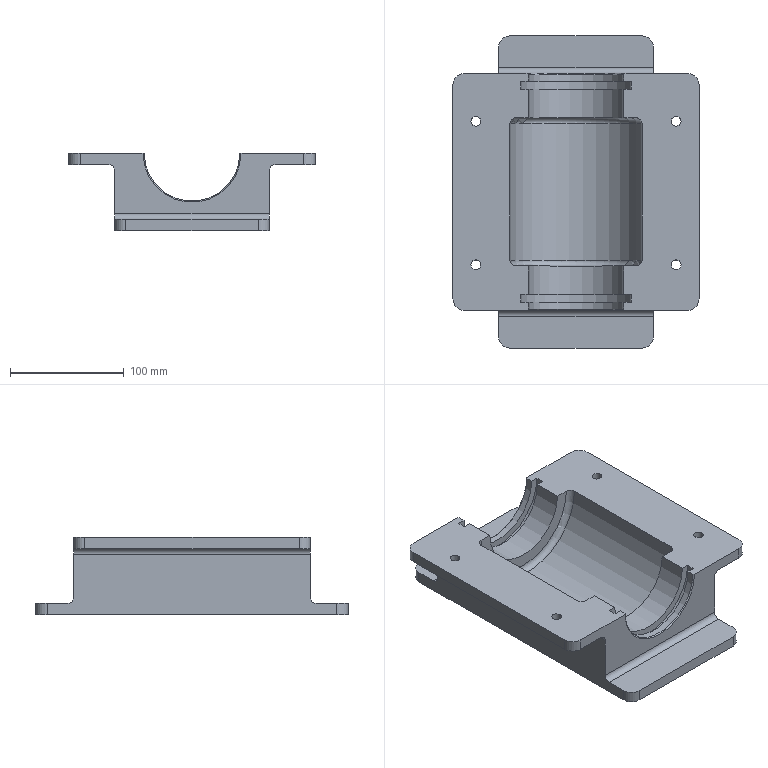Part | NX | features DATUM_CSYS 8, SKETCH 7, EXTRACT_FACE 4, HOLE PACKAGE 4, SIMPLE HOLE 4, SYMBOLIC_THREAD 4, Instance Feature 3, BLEND 2, EXTRUDE 2, CHAMFER 1, DATUM_PLANE 1, Pattern Feature 1, SWP104 1, UNITE 1 | 1 solid | 48 faces | box 216 x 274 x 68 mm | volume 1265227 mm3 | cylinder 23 | plane 21 | torus 2 | cone 2 | commonest cylinder face diameters 20 x8 8.5 x4 10 x4 84 x4 97 x2 116 x1
STEP:
#1=CARTESIAN_POINT('',(-24.25,199.,68.));
#2=VERTEX_POINT('',#1);
#3=CARTESIAN_POINT('',(-20.,199.,68.));
#4=DIRECTION('',(0.,0.,-1.));
#5=DIRECTION('',(-1.,0.,0.));
#6=AXIS2_PLACEMENT_3D('',#3,#4,#5);
#7=CIRCLE('',#6,4.25);
#8=EDGE_CURVE('',#2,#2,#7,.T.);
#9=ORIENTED_EDGE('',*,*,#8,.T.);
#10=EDGE_LOOP('',(#9));
#11=FACE_BOUND('',#10,.T.);
#12=CARTESIAN_POINT('',(-24.25,73.,68.));
#13=VERTEX_POINT('',#12);
#14=CARTESIAN_POINT('',(-20.,73.,68.));
#15=DIRECTION('',(0.,0.,-1.));
#16=DIRECTION('',(-1.,0.,0.));
#17=AXIS2_PLACEMENT_3D('',#14,#15,#16);
#18=CIRCLE('',#17,4.25);
#19=EDGE_CURVE('',#13,#13,#18,.T.);
#20=ORIENTED_EDGE('',*,*,#19,.T.);
#21=EDGE_LOOP('',(#20));
#22=FACE_BOUND('',#21,.T.);
#23=CARTESIAN_POINT('',(26.,240.,68.));
#24=VERTEX_POINT('',#23);
#25=CARTESIAN_POINT('',(26.,234.,68.));
#26=VERTEX_POINT('',#25);
#27=CARTESIAN_POINT('',(26.,33.,68.));
#28=DIRECTION('',(0.,-1.,0.));
#29=VECTOR('',#28,1000.);
#30=LINE('',#27,#29);
#31=EDGE_CURVE('',#24,#26,#30,.T.);
#32=ORIENTED_EDGE('',*,*,#31,.F.);
#33=CARTESIAN_POINT('',(25.,241.,68.));
#34=VERTEX_POINT('',#33);
#35=CARTESIAN_POINT('',(68.,198.,68.));
#36=DIRECTION('',(0.7071,-0.7071,0.));
#37=VECTOR('',#36,1000.);
#38=LINE('',#35,#37);
#39=EDGE_CURVE('',#24,#34,#38,.F.);
#40=ORIENTED_EDGE('',*,*,#39,.T.);
#41=CARTESIAN_POINT('',(-30.,241.,68.));
#42=VERTEX_POINT('',#41);
#43=CARTESIAN_POINT('',(176.,241.,68.));
#44=DIRECTION('',(-1.,0.,0.));
#45=VECTOR('',#44,1000.);
#46=LINE('',#43,#45);
#47=EDGE_CURVE('',#34,#42,#46,.T.);
#48=ORIENTED_EDGE('',*,*,#47,.T.);
#49=CARTESIAN_POINT('',(-40.,231.,68.));
#50=VERTEX_POINT('',#49);
#51=CARTESIAN_POINT('',(-30.,231.,68.));
#52=DIRECTION('',(0.,0.,1.));
#53=DIRECTION('',(1.,0.,0.));
#54=AXIS2_PLACEMENT_3D('',#51,#52,#53);
#55=CIRCLE('',#54,10.);
#56=EDGE_CURVE('',#42,#50,#55,.T.);
#57=ORIENTED_EDGE('',*,*,#56,.T.);
#58=CARTESIAN_POINT('',(-40.,43.,68.));
#59=VERTEX_POINT('',#58);
#60=CARTESIAN_POINT('',(-40.,241.,68.));
#61=DIRECTION('',(0.,-1.,0.));
#62=VECTOR('',#61,1000.);
#63=LINE('',#60,#62);
#64=EDGE_CURVE('',#50,#59,#63,.T.);
#65=ORIENTED_EDGE('',*,*,#64,.T.);
#66=CARTESIAN_POINT('',(-30.,33.,68.));
#67=VERTEX_POINT('',#66);
#68=CARTESIAN_POINT('',(-30.,43.,68.));
#69=DIRECTION('',(0.,0.,1.));
#70=DIRECTION('',(1.,0.,0.));
#71=AXIS2_PLACEMENT_3D('',#68,#69,#70);
#72=CIRCLE('',#71,10.);
#73=EDGE_CURVE('',#59,#67,#72,.T.);
#74=ORIENTED_EDGE('',*,*,#73,.T.);
#75=CARTESIAN_POINT('',(25.,33.,68.));
#76=VERTEX_POINT('',#75);
#77=CARTESIAN_POINT('',(176.,33.,68.));
#78=DIRECTION('',(-1.,0.,0.));
#79=VECTOR('',#78,1000.);
#80=LINE('',#77,#79);
#81=EDGE_CURVE('',#76,#67,#80,.T.);
#82=ORIENTED_EDGE('',*,*,#81,.F.);
#83=CARTESIAN_POINT('',(26.,34.,68.));
#84=VERTEX_POINT('',#83);
#85=CARTESIAN_POINT('',(68.,76.,68.));
#86=DIRECTION('',(-0.7071,-0.7071,0.));
#87=VECTOR('',#86,1000.);
#88=LINE('',#85,#87);
#89=EDGE_CURVE('',#76,#84,#88,.F.);
#90=ORIENTED_EDGE('',*,*,#89,.T.);
#91=CARTESIAN_POINT('',(26.,40.,68.));
#92=VERTEX_POINT('',#91);
#93=CARTESIAN_POINT('',(26.,33.,68.));
#94=DIRECTION('',(0.,-1.,0.));
#95=VECTOR('',#94,1000.);
#96=LINE('',#93,#95);
#97=EDGE_CURVE('',#92,#84,#96,.T.);
#98=ORIENTED_EDGE('',*,*,#97,.F.);
#99=CARTESIAN_POINT('',(19.5,40.,68.));
#100=VERTEX_POINT('',#99);
#101=CARTESIAN_POINT('',(176.,40.,68.));
#102=DIRECTION('',(1.,0.,0.));
#103=VECTOR('',#102,1000.);
#104=LINE('',#101,#103);
#105=EDGE_CURVE('',#100,#92,#104,.T.);
#106=ORIENTED_EDGE('',*,*,#105,.F.);
#107=CARTESIAN_POINT('',(19.5,47.,68.));
#108=VERTEX_POINT('',#107);
#109=CARTESIAN_POINT('',(19.5,33.,68.));
#110=DIRECTION('',(0.,-1.,0.));
#111=VECTOR('',#110,1000.);
#112=LINE('',#109,#111);
#113=EDGE_CURVE('',#108,#100,#112,.T.);
#114=ORIENTED_EDGE('',*,*,#113,.F.);
#115=CARTESIAN_POINT('',(26.,47.,68.));
#116=VERTEX_POINT('',#115);
#117=CARTESIAN_POINT('',(176.,47.,68.));
#118=DIRECTION('',(-1.,0.,0.));
#119=VECTOR('',#118,1000.);
#120=LINE('',#117,#119);
#121=EDGE_CURVE('',#116,#108,#120,.T.);
#122=ORIENTED_EDGE('',*,*,#121,.F.);
#123=CARTESIAN_POINT('',(26.,72.,68.));
#124=VERTEX_POINT('',#123);
#125=CARTESIAN_POINT('',(26.,33.,68.));
#126=DIRECTION('',(0.,-1.,0.));
#127=VECTOR('',#126,1000.);
#128=LINE('',#125,#127);
#129=EDGE_CURVE('',#124,#116,#128,.T.);
#130=ORIENTED_EDGE('',*,*,#129,.F.);
#131=CARTESIAN_POINT('',(15.,72.,68.));
#132=VERTEX_POINT('',#131);
#133=CARTESIAN_POINT('',(176.,72.,68.));
#134=DIRECTION('',(1.,0.,0.));
#135=VECTOR('',#134,1000.);
#136=LINE('',#133,#135);
#137=EDGE_CURVE('',#132,#124,#136,.T.);
#138=ORIENTED_EDGE('',*,*,#137,.F.);
#139=CARTESIAN_POINT('',(10.,77.,68.));
#140=VERTEX_POINT('',#139);
#141=CARTESIAN_POINT('',(15.,77.,68.));
#142=DIRECTION('',(0.,0.,1.));
#143=DIRECTION('',(1.,0.,0.));
#144=AXIS2_PLACEMENT_3D('',#141,#142,#143);
#145=CIRCLE('',#144,5.);
#146=EDGE_CURVE('',#132,#140,#145,.F.);
#147=ORIENTED_EDGE('',*,*,#146,.T.);
#148=CARTESIAN_POINT('',(10.,197.,68.));
#149=VERTEX_POINT('',#148);
#150=CARTESIAN_POINT('',(10.,33.,68.));
#151=DIRECTION('',(0.,-1.,0.));
#152=VECTOR('',#151,1000.);
#153=LINE('',#150,#152);
#154=EDGE_CURVE('',#149,#140,#153,.T.);
#155=ORIENTED_EDGE('',*,*,#154,.F.);
#156=CARTESIAN_POINT('',(15.,202.,68.));
#157=VERTEX_POINT('',#156);
#158=CARTESIAN_POINT('',(15.,197.,68.));
#159=DIRECTION('',(0.,0.,1.));
#160=DIRECTION('',(1.,0.,0.));
#161=AXIS2_PLACEMENT_3D('',#158,#159,#160);
#162=CIRCLE('',#161,5.);
#163=EDGE_CURVE('',#149,#157,#162,.F.);
#164=ORIENTED_EDGE('',*,*,#163,.T.);
#165=CARTESIAN_POINT('',(26.,202.,68.));
#166=VERTEX_POINT('',#165);
#167=CARTESIAN_POINT('',(176.,202.,68.));
#168=DIRECTION('',(-1.,0.,0.));
#169=VECTOR('',#168,1000.);
#170=LINE('',#167,#169);
#171=EDGE_CURVE('',#166,#157,#170,.T.);
#172=ORIENTED_EDGE('',*,*,#171,.F.);
#173=CARTESIAN_POINT('',(26.,227.,68.));
#174=VERTEX_POINT('',#173);
#175=CARTESIAN_POINT('',(26.,33.,68.));
#176=DIRECTION('',(0.,-1.,0.));
#177=VECTOR('',#176,1000.);
#178=LINE('',#175,#177);
#179=EDGE_CURVE('',#174,#166,#178,.T.);
#180=ORIENTED_EDGE('',*,*,#179,.F.);
#181=CARTESIAN_POINT('',(19.5,227.,68.));
#182=VERTEX_POINT('',#181);
#183=CARTESIAN_POINT('',(176.,227.,68.));
#184=DIRECTION('',(1.,0.,0.));
#185=VECTOR('',#184,1000.);
#186=LINE('',#183,#185);
#187=EDGE_CURVE('',#182,#174,#186,.T.);
#188=ORIENTED_EDGE('',*,*,#187,.F.);
#189=CARTESIAN_POINT('',(19.5,234.,68.));
#190=VERTEX_POINT('',#189);
#191=CARTESIAN_POINT('',(19.5,33.,68.));
#192=DIRECTION('',(0.,-1.,0.));
#193=VECTOR('',#192,1000.);
#194=LINE('',#191,#193);
#195=EDGE_CURVE('',#190,#182,#194,.T.);
#196=ORIENTED_EDGE('',*,*,#195,.F.);
#197=CARTESIAN_POINT('',(176.,234.,68.));
#198=DIRECTION('',(-1.,0.,0.));
#199=VECTOR('',#198,1000.);
#200=LINE('',#197,#199);
#201=EDGE_CURVE('',#26,#190,#200,.T.);
#202=ORIENTED_EDGE('',*,*,#201,.F.);
#203=EDGE_LOOP('',(#32,#40,#48,#57,#65,#74,#82,#90,#98,#106,#114,#122,#130,#138,#147,#155,#164,#172,#180,#188,#196,#202));
#204=FACE_BOUND('',#203,.T.);
#205=CARTESIAN_POINT('',(176.,241.,68.));
#206=DIRECTION('',(0.,0.,1.));
#207=DIRECTION('',(1.,0.,0.));
#208=AXIS2_PLACEMENT_3D('',#205,#206,#207);
#209=PLANE('',#208);
#210=ADVANCED_FACE('',(#11,#22,#204),#209,.T.);
#211=CARTESIAN_POINT('',(-40.,231.,58.));
#212=VERTEX_POINT('',#211);
#213=CARTESIAN_POINT('',(-40.,43.,58.));
#214=VERTEX_POINT('',#213);
#215=CARTESIAN_POINT('',(-40.,241.,58.));
#216=DIRECTION('',(0.,-1.,0.));
#217=VECTOR('',#216,1000.);
#218=LINE('',#215,#217);
#219=EDGE_CURVE('',#212,#214,#218,.T.);
#220=ORIENTED_EDGE('',*,*,#219,.T.);
#221=CARTESIAN_POINT('',(-40.,43.,68.));
#222=DIRECTION('',(0.,0.,-1.));
#223=VECTOR('',#222,1000.);
#224=LINE('',#221,#223);
#225=EDGE_CURVE('',#214,#59,#224,.F.);
#226=ORIENTED_EDGE('',*,*,#225,.T.);
#227=ORIENTED_EDGE('',*,*,#64,.F.);
#228=CARTESIAN_POINT('',(-40.,231.,58.));
#229=DIRECTION('',(0.,0.,-1.));
#230=VECTOR('',#229,1000.);
#231=LINE('',#228,#230);
#232=EDGE_CURVE('',#50,#212,#231,.T.);
#233=ORIENTED_EDGE('',*,*,#232,.T.);
#234=EDGE_LOOP('',(#220,#226,#227,#233));
#235=FACE_BOUND('',#234,.T.);
#236=CARTESIAN_POINT('',(-40.,241.,68.));
#237=DIRECTION('',(-1.,0.,0.));
#238=DIRECTION('',(0.,0.,1.));
#239=AXIS2_PLACEMENT_3D('',#236,#237,#238);
#240=PLANE('',#239);
#241=ADVANCED_FACE('',(#235),#240,.T.);
#242=CARTESIAN_POINT('',(-24.25,199.,58.));
#243=VERTEX_POINT('',#242);
#244=CARTESIAN_POINT('',(-20.,199.,58.));
#245=DIRECTION('',(0.,0.,-1.));
#246=DIRECTION('',(-1.,0.,0.));
#247=AXIS2_PLACEMENT_3D('',#244,#245,#246);
#248=CIRCLE('',#247,4.25);
#249=EDGE_CURVE('',#243,#243,#248,.T.);
#250=ORIENTED_EDGE('',*,*,#249,.F.);
#251=EDGE_LOOP('',(#250));
#252=FACE_BOUND('',#251,.T.);
#253=CARTESIAN_POINT('',(-24.25,73.,58.));
#254=VERTEX_POINT('',#253);
#255=CARTESIAN_POINT('',(-20.,73.,58.));
#256=DIRECTION('',(0.,0.,-1.));
#257=DIRECTION('',(-1.,0.,0.));
#258=AXIS2_PLACEMENT_3D('',#255,#256,#257);
#259=CIRCLE('',#258,4.25);
#260=EDGE_CURVE('',#254,#254,#259,.T.);
#261=ORIENTED_EDGE('',*,*,#260,.F.);
#262=EDGE_LOOP('',(#261));
#263=FACE_BOUND('',#262,.T.);
#264=CARTESIAN_POINT('',(-30.,241.,58.));
#265=VERTEX_POINT('',#264);
#266=CARTESIAN_POINT('',(-5.,241.,58.));
#267=VERTEX_POINT('',#266);
#268=CARTESIAN_POINT('',(-40.,241.,58.));
#269=DIRECTION('',(1.,0.,0.));
#270=VECTOR('',#269,1000.);
#271=LINE('',#268,#270);
#272=EDGE_CURVE('',#265,#267,#271,.T.);
#273=ORIENTED_EDGE('',*,*,#272,.T.);
#274=CARTESIAN_POINT('',(-5.,33.,58.));
#275=VERTEX_POINT('',#274);
#276=CARTESIAN_POINT('',(-5.,33.,58.));
#277=DIRECTION('',(0.,-1.,0.));
#278=VECTOR('',#277,1000.);
#279=LINE('',#276,#278);
#280=EDGE_CURVE('',#267,#275,#279,.T.);
#281=ORIENTED_EDGE('',*,*,#280,.T.);
#282=CARTESIAN_POINT('',(-30.,33.,58.));
#283=VERTEX_POINT('',#282);
#284=CARTESIAN_POINT('',(-40.,33.,58.));
#285=DIRECTION('',(1.,0.,0.));
#286=VECTOR('',#285,1000.);
#287=LINE('',#284,#286);
#288=EDGE_CURVE('',#283,#275,#287,.T.);
#289=ORIENTED_EDGE('',*,*,#288,.F.);
#290=CARTESIAN_POINT('',(-30.,43.,58.));
#291=DIRECTION('',(0.,0.,-1.));
#292=DIRECTION('',(-1.,0.,0.));
#293=AXIS2_PLACEMENT_3D('',#290,#291,#292);
#294=CIRCLE('',#293,10.);
#295=EDGE_CURVE('',#283,#214,#294,.T.);
#296=ORIENTED_EDGE('',*,*,#295,.T.);
#297=ORIENTED_EDGE('',*,*,#219,.F.);
#298=CARTESIAN_POINT('',(-30.,231.,58.));
#299=DIRECTION('',(0.,0.,-1.));
#300=DIRECTION('',(-1.,0.,0.));
#301=AXIS2_PLACEMENT_3D('',#298,#299,#300);
#302=CIRCLE('',#301,10.);
#303=EDGE_CURVE('',#212,#265,#302,.T.);
#304=ORIENTED_EDGE('',*,*,#303,.T.);
#305=EDGE_LOOP('',(#273,#281,#289,#296,#297,#304));
#306=FACE_BOUND('',#305,.T.);
#307=CARTESIAN_POINT('',(-40.,241.,58.));
#308=DIRECTION('',(0.,0.,-1.));
#309=DIRECTION('',(-1.,0.,0.));
#310=AXIS2_PLACEMENT_3D('',#307,#308,#309);
#311=PLANE('',#310);
#312=ADVANCED_FACE('',(#252,#263,#306),#311,.T.);
#313=CARTESIAN_POINT('',(0.,33.,53.));
#314=VERTEX_POINT('',#313);
#315=CARTESIAN_POINT('',(0.,33.,15.));
#316=VERTEX_POINT('',#315);
#317=CARTESIAN_POINT('',(0.,33.,58.));
#318=DIRECTION('',(0.,0.,-1.));
#319=VECTOR('',#318,1000.);
#320=LINE('',#317,#319);
#321=EDGE_CURVE('',#314,#316,#320,.T.);
#322=ORIENTED_EDGE('',*,*,#321,.F.);
#323=CARTESIAN_POINT('',(0.,241.,53.));
#324=VERTEX_POINT('',#323);
#325=CARTESIAN_POINT('',(0.,241.,53.));
#326=DIRECTION('',(0.,-1.,0.));
#327=VECTOR('',#326,1000.);
#328=LINE('',#325,#327);
#329=EDGE_CURVE('',#314,#324,#328,.F.);
#330=ORIENTED_EDGE('',*,*,#329,.T.);
#331=CARTESIAN_POINT('',(0.,241.,15.));
#332=VERTEX_POINT('',#331);
#333=CARTESIAN_POINT('',(0.,241.,58.));
#334=DIRECTION('',(0.,0.,-1.));
#335=VECTOR('',#334,1000.);
#336=LINE('',#333,#335);
#337=EDGE_CURVE('',#324,#332,#336,.T.);
#338=ORIENTED_EDGE('',*,*,#337,.T.);
#339=CARTESIAN_POINT('',(0.,246.,10.));
#340=VERTEX_POINT('',#339);
#341=CARTESIAN_POINT('',(0.,246.,15.));
#342=DIRECTION('',(-1.,0.,0.));
#343=DIRECTION('',(0.,0.,1.));
#344=AXIS2_PLACEMENT_3D('',#341,#342,#343);
#345=CIRCLE('',#344,5.);
#346=EDGE_CURVE('',#332,#340,#345,.F.);
#347=ORIENTED_EDGE('',*,*,#346,.T.);
#348=CARTESIAN_POINT('',(0.,264.,10.));
#349=VERTEX_POINT('',#348);
#350=CARTESIAN_POINT('',(0.,274.,10.));
#351=DIRECTION('',(0.,-1.,0.));
#352=VECTOR('',#351,1000.);
#353=LINE('',#350,#352);
#354=EDGE_CURVE('',#349,#340,#353,.T.);
#355=ORIENTED_EDGE('',*,*,#354,.F.);
#356=CARTESIAN_POINT('',(0.,264.,0.));
#357=VERTEX_POINT('',#356);
#358=CARTESIAN_POINT('',(0.,264.,0.));
#359=DIRECTION('',(0.,0.,-1.));
#360=VECTOR('',#359,1000.);
#361=LINE('',#358,#360);
#362=EDGE_CURVE('',#349,#357,#361,.T.);
#363=ORIENTED_EDGE('',*,*,#362,.T.);
#364=CARTESIAN_POINT('',(0.,10.,0.));
#365=VERTEX_POINT('',#364);
#366=CARTESIAN_POINT('',(0.,274.,0.));
#367=DIRECTION('',(0.,-1.,0.));
#368=VECTOR('',#367,1000.);
#369=LINE('',#366,#368);
#370=EDGE_CURVE('',#357,#365,#369,.T.);
#371=ORIENTED_EDGE('',*,*,#370,.T.);
#372=CARTESIAN_POINT('',(0.,10.,10.));
#373=VERTEX_POINT('',#372);
#374=CARTESIAN_POINT('',(0.,10.,10.));
#375=DIRECTION('',(0.,0.,-1.));
#376=VECTOR('',#375,1000.);
#377=LINE('',#374,#376);
#378=EDGE_CURVE('',#365,#373,#377,.F.);
#379=ORIENTED_EDGE('',*,*,#378,.T.);
#380=CARTESIAN_POINT('',(0.,28.,10.));
#381=VERTEX_POINT('',#380);
#382=CARTESIAN_POINT('',(0.,274.,10.));
#383=DIRECTION('',(0.,-1.,0.));
#384=VECTOR('',#383,1000.);
#385=LINE('',#382,#384);
#386=EDGE_CURVE('',#381,#373,#385,.T.);
#387=ORIENTED_EDGE('',*,*,#386,.F.);
#388=CARTESIAN_POINT('',(0.,28.,15.));
#389=DIRECTION('',(-1.,0.,0.));
#390=DIRECTION('',(0.,0.,1.));
#391=AXIS2_PLACEMENT_3D('',#388,#389,#390);
#392=CIRCLE('',#391,5.);
#393=EDGE_CURVE('',#381,#316,#392,.F.);
#394=ORIENTED_EDGE('',*,*,#393,.T.);
#395=EDGE_LOOP('',(#322,#330,#338,#347,#355,#363,#371,#379,#387,#394));
#396=FACE_BOUND('',#395,.T.);
#397=CARTESIAN_POINT('',(0.,241.,58.));
#398=DIRECTION('',(-1.,0.,0.));
#399=DIRECTION('',(0.,0.,1.));
#400=AXIS2_PLACEMENT_3D('',#397,#398,#399);
#401=PLANE('',#400);
#402=ADVANCED_FACE('',(#396),#401,.T.);
#403=CARTESIAN_POINT('',(136.,241.,15.));
#404=VERTEX_POINT('',#403);
#405=CARTESIAN_POINT('',(136.,241.,53.));
#406=VERTEX_POINT('',#405);
#407=CARTESIAN_POINT('',(136.,241.,10.));
#408=DIRECTION('',(0.,0.,1.));
#409=VECTOR('',#408,1000.);
#410=LINE('',#407,#409);
#411=EDGE_CURVE('',#404,#406,#410,.T.);
#412=ORIENTED_EDGE('',*,*,#411,.T.);
#413=CARTESIAN_POINT('',(136.,33.,53.));
#414=VERTEX_POINT('',#413);
#415=CARTESIAN_POINT('',(136.,33.,53.));
#416=DIRECTION('',(0.,-1.,0.));
#417=VECTOR('',#416,1000.);
#418=LINE('',#415,#417);
#419=EDGE_CURVE('',#406,#414,#418,.T.);
#420=ORIENTED_EDGE('',*,*,#419,.T.);
#421=CARTESIAN_POINT('',(136.,33.,15.));
#422=VERTEX_POINT('',#421);
#423=CARTESIAN_POINT('',(136.,33.,10.));
#424=DIRECTION('',(0.,0.,1.));
#425=VECTOR('',#424,1000.);
#426=LINE('',#423,#425);
#427=EDGE_CURVE('',#422,#414,#426,.T.);
#428=ORIENTED_EDGE('',*,*,#427,.F.);
#429=CARTESIAN_POINT('',(136.,28.,10.));
#430=VERTEX_POINT('',#429);
#431=CARTESIAN_POINT('',(136.,28.,15.));
#432=DIRECTION('',(1.,0.,0.));
#433=DIRECTION('',(0.,0.,-1.));
#434=AXIS2_PLACEMENT_3D('',#431,#432,#433);
#435=CIRCLE('',#434,5.);
#436=EDGE_CURVE('',#422,#430,#435,.F.);
#437=ORIENTED_EDGE('',*,*,#436,.T.);
#438=CARTESIAN_POINT('',(136.,10.,10.));
#439=VERTEX_POINT('',#438);
#440=CARTESIAN_POINT('',(136.,0.,10.));
#441=DIRECTION('',(0.,1.,0.));
#442=VECTOR('',#441,1000.);
#443=LINE('',#440,#442);
#444=EDGE_CURVE('',#439,#430,#443,.T.);
#445=ORIENTED_EDGE('',*,*,#444,.F.);
#446=CARTESIAN_POINT('',(136.,10.,0.));
#447=VERTEX_POINT('',#446);
#448=CARTESIAN_POINT('',(136.,10.,0.));
#449=DIRECTION('',(0.,0.,-1.));
#450=VECTOR('',#449,1000.);
#451=LINE('',#448,#450);
#452=EDGE_CURVE('',#439,#447,#451,.T.);
#453=ORIENTED_EDGE('',*,*,#452,.T.);
#454=CARTESIAN_POINT('',(136.,264.,0.));
#455=VERTEX_POINT('',#454);
#456=CARTESIAN_POINT('',(136.,0.,0.));
#457=DIRECTION('',(0.,1.,0.));
#458=VECTOR('',#457,1000.);
#459=LINE('',#456,#458);
#460=EDGE_CURVE('',#447,#455,#459,.T.);
#461=ORIENTED_EDGE('',*,*,#460,.T.);
#462=CARTESIAN_POINT('',(136.,264.,10.));
#463=VERTEX_POINT('',#462);
#464=CARTESIAN_POINT('',(136.,264.,10.));
#465=DIRECTION('',(0.,0.,-1.));
#466=VECTOR('',#465,1000.);
#467=LINE('',#464,#466);
#468=EDGE_CURVE('',#455,#463,#467,.F.);
#469=ORIENTED_EDGE('',*,*,#468,.T.);
#470=CARTESIAN_POINT('',(136.,246.,10.));
#471=VERTEX_POINT('',#470);
#472=CARTESIAN_POINT('',(136.,0.,10.));
#473=DIRECTION('',(0.,1.,0.));
#474=VECTOR('',#473,1000.);
#475=LINE('',#472,#474);
#476=EDGE_CURVE('',#471,#463,#475,.T.);
#477=ORIENTED_EDGE('',*,*,#476,.F.);
#478=CARTESIAN_POINT('',(136.,246.,15.));
#479=DIRECTION('',(1.,0.,0.));
#480=DIRECTION('',(0.,0.,-1.));
#481=AXIS2_PLACEMENT_3D('',#478,#479,#480);
#482=CIRCLE('',#481,5.);
#483=EDGE_CURVE('',#471,#404,#482,.F.);
#484=ORIENTED_EDGE('',*,*,#483,.T.);
#485=EDGE_LOOP('',(#412,#420,#428,#437,#445,#453,#461,#469,#477,#484));
#486=FACE_BOUND('',#485,.T.);
#487=CARTESIAN_POINT('',(136.,241.,10.));
#488=DIRECTION('',(1.,0.,0.));
#489=DIRECTION('',(0.,0.,-1.));
#490=AXIS2_PLACEMENT_3D('',#487,#488,#489);
#491=PLANE('',#490);
#492=ADVANCED_FACE('',(#486),#491,.T.);
#493=CARTESIAN_POINT('',(151.75,199.,58.));
#494=VERTEX_POINT('',#493);
#495=CARTESIAN_POINT('',(156.,199.,58.));
#496=DIRECTION('',(0.,0.,-1.));
#497=DIRECTION('',(-1.,0.,0.));
#498=AXIS2_PLACEMENT_3D('',#495,#496,#497);
#499=CIRCLE('',#498,4.25);
#500=EDGE_CURVE('',#494,#494,#499,.T.);
#501=ORIENTED_EDGE('',*,*,#500,.F.);
#502=EDGE_LOOP('',(#501));
#503=FACE_BOUND('',#502,.T.);
#504=CARTESIAN_POINT('',(151.75,73.,58.));
#505=VERTEX_POINT('',#504);
#506=CARTESIAN_POINT('',(156.,73.,58.));
#507=DIRECTION('',(0.,0.,-1.));
#508=DIRECTION('',(-1.,0.,0.));
#509=AXIS2_PLACEMENT_3D('',#506,#507,#508);
#510=CIRCLE('',#509,4.25);
#511=EDGE_CURVE('',#505,#505,#510,.T.);
#512=ORIENTED_EDGE('',*,*,#511,.F.);
#513=EDGE_LOOP('',(#512));
#514=FACE_BOUND('',#513,.T.);
#515=CARTESIAN_POINT('',(141.,33.,58.));
#516=VERTEX_POINT('',#515);
#517=CARTESIAN_POINT('',(166.,33.,58.));
#518=VERTEX_POINT('',#517);
#519=CARTESIAN_POINT('',(136.,33.,58.));
#520=DIRECTION('',(1.,0.,0.));
#521=VECTOR('',#520,1000.);
#522=LINE('',#519,#521);
#523=EDGE_CURVE('',#516,#518,#522,.T.);
#524=ORIENTED_EDGE('',*,*,#523,.F.);
#525=CARTESIAN_POINT('',(141.,241.,58.));
#526=VERTEX_POINT('',#525);
#527=CARTESIAN_POINT('',(141.,241.,58.));
#528=DIRECTION('',(0.,-1.,0.));
#529=VECTOR('',#528,1000.);
#530=LINE('',#527,#529);
#531=EDGE_CURVE('',#516,#526,#530,.F.);
#532=ORIENTED_EDGE('',*,*,#531,.T.);
#533=CARTESIAN_POINT('',(166.,241.,58.));
#534=VERTEX_POINT('',#533);
#535=CARTESIAN_POINT('',(136.,241.,58.));
#536=DIRECTION('',(1.,0.,0.));
#537=VECTOR('',#536,1000.);
#538=LINE('',#535,#537);
#539=EDGE_CURVE('',#526,#534,#538,.T.);
#540=ORIENTED_EDGE('',*,*,#539,.T.);
#541=CARTESIAN_POINT('',(176.,231.,58.));
#542=VERTEX_POINT('',#541);
#543=CARTESIAN_POINT('',(166.,231.,58.));
#544=DIRECTION('',(0.,0.,-1.));
#545=DIRECTION('',(-1.,0.,0.));
#546=AXIS2_PLACEMENT_3D('',#543,#544,#545);
#547=CIRCLE('',#546,10.);
#548=EDGE_CURVE('',#534,#542,#547,.T.);
#549=ORIENTED_EDGE('',*,*,#548,.T.);
#550=CARTESIAN_POINT('',(176.,43.,58.));
#551=VERTEX_POINT('',#550);
#552=CARTESIAN_POINT('',(176.,241.,58.));
#553=DIRECTION('',(0.,-1.,0.));
#554=VECTOR('',#553,1000.);
#555=LINE('',#552,#554);
#556=EDGE_CURVE('',#542,#551,#555,.T.);
#557=ORIENTED_EDGE('',*,*,#556,.T.);
#558=CARTESIAN_POINT('',(166.,43.,58.));
#559=DIRECTION('',(0.,0.,-1.));
#560=DIRECTION('',(-1.,0.,0.));
#561=AXIS2_PLACEMENT_3D('',#558,#559,#560);
#562=CIRCLE('',#561,10.);
#563=EDGE_CURVE('',#551,#518,#562,.T.);
#564=ORIENTED_EDGE('',*,*,#563,.T.);
#565=EDGE_LOOP('',(#524,#532,#540,#549,#557,#564));
#566=FACE_BOUND('',#565,.T.);
#567=CARTESIAN_POINT('',(136.,241.,58.));
#568=DIRECTION('',(0.,0.,-1.));
#569=DIRECTION('',(-1.,0.,0.));
#570=AXIS2_PLACEMENT_3D('',#567,#568,#569);
#571=PLANE('',#570);
#572=ADVANCED_FACE('',(#503,#514,#566),#571,.T.);
#573=CARTESIAN_POINT('',(176.,231.,68.));
#574=VERTEX_POINT('',#573);
#575=CARTESIAN_POINT('',(176.,43.,68.));
#576=VERTEX_POINT('',#575);
#577=CARTESIAN_POINT('',(176.,241.,68.));
#578=DIRECTION('',(0.,-1.,0.));
#579=VECTOR('',#578,1000.);
#580=LINE('',#577,#579);
#581=EDGE_CURVE('',#574,#576,#580,.T.);
#582=ORIENTED_EDGE('',*,*,#581,.T.);
#583=CARTESIAN_POINT('',(176.,43.,58.));
#584=DIRECTION('',(0.,0.,1.));
#585=VECTOR('',#584,1000.);
#586=LINE('',#583,#585);
#587=EDGE_CURVE('',#576,#551,#586,.F.);
#588=ORIENTED_EDGE('',*,*,#587,.T.);
#589=ORIENTED_EDGE('',*,*,#556,.F.);
#590=CARTESIAN_POINT('',(176.,231.,68.));
#591=DIRECTION('',(0.,0.,1.));
#592=VECTOR('',#591,1000.);
#593=LINE('',#590,#592);
#594=EDGE_CURVE('',#542,#574,#593,.T.);
#595=ORIENTED_EDGE('',*,*,#594,.T.);
#596=EDGE_LOOP('',(#582,#588,#589,#595));
#597=FACE_BOUND('',#596,.T.);
#598=CARTESIAN_POINT('',(176.,241.,58.));
#599=DIRECTION('',(1.,0.,0.));
#600=DIRECTION('',(0.,0.,-1.));
#601=AXIS2_PLACEMENT_3D('',#598,#599,#600);
#602=PLANE('',#601);
#603=ADVANCED_FACE('',(#597),#602,.T.);
#604=CARTESIAN_POINT('',(151.75,199.,68.));
#605=VERTEX_POINT('',#604);
#606=CARTESIAN_POINT('',(156.,199.,68.));
#607=DIRECTION('',(0.,0.,-1.));
#608=DIRECTION('',(-1.,0.,0.));
#609=AXIS2_PLACEMENT_3D('',#606,#607,#608);
#610=CIRCLE('',#609,4.25);
#611=EDGE_CURVE('',#605,#605,#610,.T.);
#612=ORIENTED_EDGE('',*,*,#611,.T.);
#613=EDGE_LOOP('',(#612));
#614=FACE_BOUND('',#613,.T.);
#615=CARTESIAN_POINT('',(151.75,73.,68.));
#616=VERTEX_POINT('',#615);
#617=CARTESIAN_POINT('',(156.,73.,68.));
#618=DIRECTION('',(0.,0.,-1.));
#619=DIRECTION('',(-1.,0.,0.));
#620=AXIS2_PLACEMENT_3D('',#617,#618,#619);
#621=CIRCLE('',#620,4.25);
#622=EDGE_CURVE('',#616,#616,#621,.T.);
#623=ORIENTED_EDGE('',*,*,#622,.T.);
#624=EDGE_LOOP('',(#623));
#625=FACE_BOUND('',#624,.T.);
#626=CARTESIAN_POINT('',(166.,241.,68.));
#627=VERTEX_POINT('',#626);
#628=CARTESIAN_POINT('',(111.,241.,68.));
#629=VERTEX_POINT('',#628);
#630=CARTESIAN_POINT('',(176.,241.,68.));
#631=DIRECTION('',(-1.,0.,0.));
#632=VECTOR('',#631,1000.);
#633=LINE('',#630,#632);
#634=EDGE_CURVE('',#627,#629,#633,.T.);
#635=ORIENTED_EDGE('',*,*,#634,.T.);
#636=CARTESIAN_POINT('',(110.,240.,68.));
#637=VERTEX_POINT('',#636);
#638=CARTESIAN_POINT('',(68.,198.,68.));
#639=DIRECTION('',(0.7071,0.7071,0.));
#640=VECTOR('',#639,1000.);
#641=LINE('',#638,#640);
#642=EDGE_CURVE('',#629,#637,#641,.F.);
#643=ORIENTED_EDGE('',*,*,#642,.T.);
#644=CARTESIAN_POINT('',(110.,234.,68.));
#645=VERTEX_POINT('',#644);
#646=CARTESIAN_POINT('',(110.,33.,68.));
#647=DIRECTION('',(0.,-1.,0.));
#648=VECTOR('',#647,1000.);
#649=LINE('',#646,#648);
#650=EDGE_CURVE('',#645,#637,#649,.F.);
#651=ORIENTED_EDGE('',*,*,#650,.F.);
#652=CARTESIAN_POINT('',(116.5,234.,68.));
#653=VERTEX_POINT('',#652);
#654=CARTESIAN_POINT('',(176.,234.,68.));
#655=DIRECTION('',(-1.,0.,0.));
#656=VECTOR('',#655,1000.);
#657=LINE('',#654,#656);
#658=EDGE_CURVE('',#653,#645,#657,.T.);
#659=ORIENTED_EDGE('',*,*,#658,.F.);
#660=CARTESIAN_POINT('',(116.5,227.,68.));
#661=VERTEX_POINT('',#660);
#662=CARTESIAN_POINT('',(116.5,33.,68.));
#663=DIRECTION('',(0.,-1.,0.));
#664=VECTOR('',#663,1000.);
#665=LINE('',#662,#664);
#666=EDGE_CURVE('',#661,#653,#665,.F.);
#667=ORIENTED_EDGE('',*,*,#666,.F.);
#668=CARTESIAN_POINT('',(110.,227.,68.));
#669=VERTEX_POINT('',#668);
#670=CARTESIAN_POINT('',(176.,227.,68.));
#671=DIRECTION('',(1.,0.,0.));
#672=VECTOR('',#671,1000.);
#673=LINE('',#670,#672);
#674=EDGE_CURVE('',#669,#661,#673,.T.);
#675=ORIENTED_EDGE('',*,*,#674,.F.);
#676=CARTESIAN_POINT('',(110.,202.,68.));
#677=VERTEX_POINT('',#676);
#678=CARTESIAN_POINT('',(110.,33.,68.));
#679=DIRECTION('',(0.,-1.,0.));
#680=VECTOR('',#679,1000.);
#681=LINE('',#678,#680);
#682=EDGE_CURVE('',#677,#669,#681,.F.);
#683=ORIENTED_EDGE('',*,*,#682,.F.);
#684=CARTESIAN_POINT('',(121.,202.,68.));
#685=VERTEX_POINT('',#684);
#686=CARTESIAN_POINT('',(176.,202.,68.));
#687=DIRECTION('',(-1.,0.,0.));
#688=VECTOR('',#687,1000.);
#689=LINE('',#686,#688);
#690=EDGE_CURVE('',#685,#677,#689,.T.);
#691=ORIENTED_EDGE('',*,*,#690,.F.);
#692=CARTESIAN_POINT('',(126.,197.,68.));
#693=VERTEX_POINT('',#692);
#694=CARTESIAN_POINT('',(121.,197.,68.));
#695=DIRECTION('',(0.,0.,1.));
#696=DIRECTION('',(1.,0.,0.));
#697=AXIS2_PLACEMENT_3D('',#694,#695,#696);
#698=CIRCLE('',#697,5.);
#699=EDGE_CURVE('',#685,#693,#698,.F.);
#700=ORIENTED_EDGE('',*,*,#699,.T.);
#701=CARTESIAN_POINT('',(126.,77.,68.));
#702=VERTEX_POINT('',#701);
#703=CARTESIAN_POINT('',(126.,33.,68.));
#704=DIRECTION('',(0.,-1.,0.));
#705=VECTOR('',#704,1000.);
#706=LINE('',#703,#705);
#707=EDGE_CURVE('',#702,#693,#706,.F.);
#708=ORIENTED_EDGE('',*,*,#707,.F.);
#709=CARTESIAN_POINT('',(121.,72.,68.));
#710=VERTEX_POINT('',#709);
#711=CARTESIAN_POINT('',(121.,77.,68.));
#712=DIRECTION('',(0.,0.,1.));
#713=DIRECTION('',(1.,0.,0.));
#714=AXIS2_PLACEMENT_3D('',#711,#712,#713);
#715=CIRCLE('',#714,5.);
#716=EDGE_CURVE('',#702,#710,#715,.F.);
#717=ORIENTED_EDGE('',*,*,#716,.T.);
#718=CARTESIAN_POINT('',(110.,72.,68.));
#719=VERTEX_POINT('',#718);
#720=CARTESIAN_POINT('',(176.,72.,68.));
#721=DIRECTION('',(1.,0.,0.));
#722=VECTOR('',#721,1000.);
#723=LINE('',#720,#722);
#724=EDGE_CURVE('',#719,#710,#723,.T.);
#725=ORIENTED_EDGE('',*,*,#724,.F.);
#726=CARTESIAN_POINT('',(110.,47.,68.));
#727=VERTEX_POINT('',#726);
#728=CARTESIAN_POINT('',(110.,33.,68.));
#729=DIRECTION('',(0.,-1.,0.));
#730=VECTOR('',#729,1000.);
#731=LINE('',#728,#730);
#732=EDGE_CURVE('',#727,#719,#731,.F.);
#733=ORIENTED_EDGE('',*,*,#732,.F.);
#734=CARTESIAN_POINT('',(116.5,47.,68.));
#735=VERTEX_POINT('',#734);
#736=CARTESIAN_POINT('',(176.,47.,68.));
#737=DIRECTION('',(-1.,0.,0.));
#738=VECTOR('',#737,1000.);
#739=LINE('',#736,#738);
#740=EDGE_CURVE('',#735,#727,#739,.T.);
#741=ORIENTED_EDGE('',*,*,#740,.F.);
#742=CARTESIAN_POINT('',(116.5,40.,68.));
#743=VERTEX_POINT('',#742);
#744=CARTESIAN_POINT('',(116.5,33.,68.));
#745=DIRECTION('',(0.,-1.,0.));
#746=VECTOR('',#745,1000.);
#747=LINE('',#744,#746);
#748=EDGE_CURVE('',#743,#735,#747,.F.);
#749=ORIENTED_EDGE('',*,*,#748,.F.);
#750=CARTESIAN_POINT('',(110.,40.,68.));
#751=VERTEX_POINT('',#750);
#752=CARTESIAN_POINT('',(176.,40.,68.));
#753=DIRECTION('',(1.,0.,0.));
#754=VECTOR('',#753,1000.);
#755=LINE('',#752,#754);
#756=EDGE_CURVE('',#751,#743,#755,.T.);
#757=ORIENTED_EDGE('',*,*,#756,.F.);
#758=CARTESIAN_POINT('',(110.,34.,68.));
#759=VERTEX_POINT('',#758);
#760=CARTESIAN_POINT('',(110.,33.,68.));
#761=DIRECTION('',(0.,-1.,0.));
#762=VECTOR('',#761,1000.);
#763=LINE('',#760,#762);
#764=EDGE_CURVE('',#759,#751,#763,.F.);
#765=ORIENTED_EDGE('',*,*,#764,.F.);
#766=CARTESIAN_POINT('',(111.,33.,68.));
#767=VERTEX_POINT('',#766);
#768=CARTESIAN_POINT('',(68.,76.,68.));
#769=DIRECTION('',(-0.7071,0.7071,0.));
#770=VECTOR('',#769,1000.);
#771=LINE('',#768,#770);
#772=EDGE_CURVE('',#759,#767,#771,.F.);
#773=ORIENTED_EDGE('',*,*,#772,.T.);
#774=CARTESIAN_POINT('',(166.,33.,68.));
#775=VERTEX_POINT('',#774);
#776=CARTESIAN_POINT('',(176.,33.,68.));
#777=DIRECTION('',(-1.,0.,0.));
#778=VECTOR('',#777,1000.);
#779=LINE('',#776,#778);
#780=EDGE_CURVE('',#775,#767,#779,.T.);
#781=ORIENTED_EDGE('',*,*,#780,.F.);
#782=CARTESIAN_POINT('',(166.,43.,68.));
#783=DIRECTION('',(0.,0.,1.));
#784=DIRECTION('',(1.,0.,0.));
#785=AXIS2_PLACEMENT_3D('',#782,#783,#784);
#786=CIRCLE('',#785,10.);
#787=EDGE_CURVE('',#775,#576,#786,.T.);
#788=ORIENTED_EDGE('',*,*,#787,.T.);
#789=ORIENTED_EDGE('',*,*,#581,.F.);
#790=CARTESIAN_POINT('',(166.,231.,68.));
#791=DIRECTION('',(0.,0.,1.));
#792=DIRECTION('',(1.,0.,0.));
#793=AXIS2_PLACEMENT_3D('',#790,#791,#792);
#794=CIRCLE('',#793,10.);
#795=EDGE_CURVE('',#574,#627,#794,.T.);
#796=ORIENTED_EDGE('',*,*,#795,.T.);
#797=EDGE_LOOP('',(#635,#643,#651,#659,#667,#675,#683,#691,#700,#708,#717,#725,#733,#741,#749,#757,#765,#773,#781,#788,#789,#796));
#798=FACE_BOUND('',#797,.T.);
#799=CARTESIAN_POINT('',(176.,241.,68.));
#800=DIRECTION('',(0.,0.,1.));
#801=DIRECTION('',(1.,0.,0.));
#802=AXIS2_PLACEMENT_3D('',#799,#800,#801);
#803=PLANE('',#802);
#804=ADVANCED_FACE('',(#614,#625,#798),#803,.T.);
#805=ORIENTED_EDGE('',*,*,#47,.F.);
#806=CARTESIAN_POINT('',(68.,241.,68.));
#807=DIRECTION('',(0.,-1.,0.));
#808=DIRECTION('',(0.,0.,-1.));
#809=AXIS2_PLACEMENT_3D('',#806,#807,#808);
#810=CIRCLE('',#809,43.);
#811=EDGE_CURVE('',#34,#629,#810,.T.);
#812=ORIENTED_EDGE('',*,*,#811,.T.);
#813=ORIENTED_EDGE('',*,*,#634,.F.);
#814=CARTESIAN_POINT('',(166.,241.,58.));
#815=DIRECTION('',(0.,0.,1.));
#816=VECTOR('',#815,1000.);
#817=LINE('',#814,#816);
#818=EDGE_CURVE('',#627,#534,#817,.F.);
#819=ORIENTED_EDGE('',*,*,#818,.T.);
#820=ORIENTED_EDGE('',*,*,#539,.F.);
#821=CARTESIAN_POINT('',(141.,241.,53.));
#822=DIRECTION('',(0.,-1.,0.));
#823=DIRECTION('',(0.,0.,-1.));
#824=AXIS2_PLACEMENT_3D('',#821,#822,#823);
#825=CIRCLE('',#824,5.);
#826=EDGE_CURVE('',#526,#406,#825,.T.);
#827=ORIENTED_EDGE('',*,*,#826,.T.);
#828=ORIENTED_EDGE('',*,*,#411,.F.);
#829=CARTESIAN_POINT('',(0.,241.,15.));
#830=DIRECTION('',(1.,0.,0.));
#831=VECTOR('',#830,1000.);
#832=LINE('',#829,#831);
#833=EDGE_CURVE('',#404,#332,#832,.F.);
#834=ORIENTED_EDGE('',*,*,#833,.T.);
#835=ORIENTED_EDGE('',*,*,#337,.F.);
#836=CARTESIAN_POINT('',(-5.,241.,53.));
#837=DIRECTION('',(0.,-1.,0.));
#838=DIRECTION('',(0.,0.,-1.));
#839=AXIS2_PLACEMENT_3D('',#836,#837,#838);
#840=CIRCLE('',#839,5.);
#841=EDGE_CURVE('',#324,#267,#840,.T.);
#842=ORIENTED_EDGE('',*,*,#841,.T.);
#843=ORIENTED_EDGE('',*,*,#272,.F.);
#844=CARTESIAN_POINT('',(-30.,241.,68.));
#845=DIRECTION('',(0.,0.,-1.));
#846=VECTOR('',#845,1000.);
#847=LINE('',#844,#846);
#848=EDGE_CURVE('',#265,#42,#847,.F.);
#849=ORIENTED_EDGE('',*,*,#848,.T.);
#850=EDGE_LOOP('',(#805,#812,#813,#819,#820,#827,#828,#834,#835,#842,#843,#849));
#851=FACE_BOUND('',#850,.T.);
#852=CARTESIAN_POINT('',(0.,241.,0.));
#853=DIRECTION('',(0.,-1.,0.));
#854=DIRECTION('',(0.,0.,-1.));
#855=AXIS2_PLACEMENT_3D('',#852,#853,#854);
#856=PLANE('',#855);
#857=ADVANCED_FACE('',(#851),#856,.F.);
#858=ORIENTED_EDGE('',*,*,#780,.T.);
#859=CARTESIAN_POINT('',(68.,33.,68.));
#860=DIRECTION('',(0.,-1.,0.));
#861=DIRECTION('',(0.,0.,-1.));
#862=AXIS2_PLACEMENT_3D('',#859,#860,#861);
#863=CIRCLE('',#862,43.);
#864=EDGE_CURVE('',#767,#76,#863,.F.);
#865=ORIENTED_EDGE('',*,*,#864,.T.);
#866=ORIENTED_EDGE('',*,*,#81,.T.);
#867=CARTESIAN_POINT('',(-30.,33.,0.));
#868=DIRECTION('',(0.,0.,-1.));
#869=VECTOR('',#868,1000.);
#870=LINE('',#867,#869);
#871=EDGE_CURVE('',#67,#283,#870,.T.);
#872=ORIENTED_EDGE('',*,*,#871,.T.);
#873=ORIENTED_EDGE('',*,*,#288,.T.);
#874=CARTESIAN_POINT('',(-5.,33.,53.));
#875=DIRECTION('',(0.,-1.,0.));
#876=DIRECTION('',(0.,0.,-1.));
#877=AXIS2_PLACEMENT_3D('',#874,#875,#876);
#878=CIRCLE('',#877,5.);
#879=EDGE_CURVE('',#275,#314,#878,.F.);
#880=ORIENTED_EDGE('',*,*,#879,.T.);
#881=ORIENTED_EDGE('',*,*,#321,.T.);
#882=CARTESIAN_POINT('',(136.,33.,15.));
#883=DIRECTION('',(1.,0.,0.));
#884=VECTOR('',#883,1000.);
#885=LINE('',#882,#884);
#886=EDGE_CURVE('',#316,#422,#885,.T.);
#887=ORIENTED_EDGE('',*,*,#886,.T.);
#888=ORIENTED_EDGE('',*,*,#427,.T.);
#889=CARTESIAN_POINT('',(141.,33.,53.));
#890=DIRECTION('',(0.,-1.,0.));
#891=DIRECTION('',(0.,0.,-1.));
#892=AXIS2_PLACEMENT_3D('',#889,#890,#891);
#893=CIRCLE('',#892,5.);
#894=EDGE_CURVE('',#414,#516,#893,.F.);
#895=ORIENTED_EDGE('',*,*,#894,.T.);
#896=ORIENTED_EDGE('',*,*,#523,.T.);
#897=CARTESIAN_POINT('',(166.,33.,0.));
#898=DIRECTION('',(0.,0.,1.));
#899=VECTOR('',#898,1000.);
#900=LINE('',#897,#899);
#901=EDGE_CURVE('',#518,#775,#900,.T.);
#902=ORIENTED_EDGE('',*,*,#901,.T.);
#903=EDGE_LOOP('',(#858,#865,#866,#872,#873,#880,#881,#887,#888,#895,#896,#902));
#904=FACE_BOUND('',#903,.T.);
#905=CARTESIAN_POINT('',(0.,33.,0.));
#906=DIRECTION('',(0.,-1.,0.));
#907=DIRECTION('',(0.,0.,-1.));
#908=AXIS2_PLACEMENT_3D('',#905,#906,#907);
#909=PLANE('',#908);
#910=ADVANCED_FACE('',(#904),#909,.T.);
#911=ORIENTED_EDGE('',*,*,#444,.T.);
#912=CARTESIAN_POINT('',(0.,28.,10.));
#913=DIRECTION('',(1.,0.,0.));
#914=VECTOR('',#913,1000.);
#915=LINE('',#912,#914);
#916=EDGE_CURVE('',#430,#381,#915,.F.);
#917=ORIENTED_EDGE('',*,*,#916,.T.);
#918=ORIENTED_EDGE('',*,*,#386,.T.);
#919=CARTESIAN_POINT('',(10.,0.,10.));
#920=VERTEX_POINT('',#919);
#921=CARTESIAN_POINT('',(10.,10.,10.));
#922=DIRECTION('',(0.,0.,1.));
#923=DIRECTION('',(1.,0.,0.));
#924=AXIS2_PLACEMENT_3D('',#921,#922,#923);
#925=CIRCLE('',#924,10.);
#926=EDGE_CURVE('',#373,#920,#925,.T.);
#927=ORIENTED_EDGE('',*,*,#926,.T.);
#928=CARTESIAN_POINT('',(126.,0.,10.));
#929=VERTEX_POINT('',#928);
#930=CARTESIAN_POINT('',(0.,0.,10.));
#931=DIRECTION('',(1.,0.,0.));
#932=VECTOR('',#931,1000.);
#933=LINE('',#930,#932);
#934=EDGE_CURVE('',#920,#929,#933,.T.);
#935=ORIENTED_EDGE('',*,*,#934,.T.);
#936=CARTESIAN_POINT('',(126.,10.,10.));
#937=DIRECTION('',(0.,0.,1.));
#938=DIRECTION('',(1.,0.,0.));
#939=AXIS2_PLACEMENT_3D('',#936,#937,#938);
#940=CIRCLE('',#939,10.);
#941=EDGE_CURVE('',#929,#439,#940,.T.);
#942=ORIENTED_EDGE('',*,*,#941,.T.);
#943=EDGE_LOOP('',(#911,#917,#918,#927,#935,#942));
#944=FACE_BOUND('',#943,.T.);
#945=CARTESIAN_POINT('',(0.,0.,10.));
#946=DIRECTION('',(0.,0.,1.));
#947=DIRECTION('',(1.,0.,0.));
#948=AXIS2_PLACEMENT_3D('',#945,#946,#947);
#949=PLANE('',#948);
#950=ADVANCED_FACE('',(#944),#949,.T.);
#951=CARTESIAN_POINT('',(10.,0.,0.));
#952=VERTEX_POINT('',#951);
#953=CARTESIAN_POINT('',(126.,0.,0.));
#954=VERTEX_POINT('',#953);
#955=CARTESIAN_POINT('',(0.,0.,0.));
#956=DIRECTION('',(1.,0.,0.));
#957=VECTOR('',#956,1000.);
#958=LINE('',#955,#957);
#959=EDGE_CURVE('',#952,#954,#958,.T.);
#960=ORIENTED_EDGE('',*,*,#959,.T.);
#961=CARTESIAN_POINT('',(126.,0.,10.));
#962=DIRECTION('',(0.,0.,-1.));
#963=VECTOR('',#962,1000.);
#964=LINE('',#961,#963);
#965=EDGE_CURVE('',#954,#929,#964,.F.);
#966=ORIENTED_EDGE('',*,*,#965,.T.);
#967=ORIENTED_EDGE('',*,*,#934,.F.);
#968=CARTESIAN_POINT('',(10.,0.,0.));
#969=DIRECTION('',(0.,0.,-1.));
#970=VECTOR('',#969,1000.);
#971=LINE('',#968,#970);
#972=EDGE_CURVE('',#920,#952,#971,.T.);
#973=ORIENTED_EDGE('',*,*,#972,.T.);
#974=EDGE_LOOP('',(#960,#966,#967,#973));
#975=FACE_BOUND('',#974,.T.);
#976=CARTESIAN_POINT('',(0.,0.,10.));
#977=DIRECTION('',(0.,1.,0.));
#978=DIRECTION('',(-1.,0.,0.));
#979=AXIS2_PLACEMENT_3D('',#976,#977,#978);
#980=PLANE('',#979);
#981=ADVANCED_FACE('',(#975),#980,.F.);
#982=CARTESIAN_POINT('',(126.,274.,0.));
#983=VERTEX_POINT('',#982);
#984=CARTESIAN_POINT('',(10.,274.,0.));
#985=VERTEX_POINT('',#984);
#986=CARTESIAN_POINT('',(136.,274.,0.));
#987=DIRECTION('',(-1.,0.,0.));
#988=VECTOR('',#987,1000.);
#989=LINE('',#986,#988);
#990=EDGE_CURVE('',#983,#985,#989,.T.);
#991=ORIENTED_EDGE('',*,*,#990,.T.);
#992=CARTESIAN_POINT('',(10.,274.,10.));
#993=VERTEX_POINT('',#992);
#994=CARTESIAN_POINT('',(10.,274.,10.));
#995=DIRECTION('',(0.,0.,-1.));
#996=VECTOR('',#995,1000.);
#997=LINE('',#994,#996);
#998=EDGE_CURVE('',#985,#993,#997,.F.);
#999=ORIENTED_EDGE('',*,*,#998,.T.);
#1000=CARTESIAN_POINT('',(126.,274.,10.));
#1001=VERTEX_POINT('',#1000);
#1002=CARTESIAN_POINT('',(136.,274.,10.));
#1003=DIRECTION('',(-1.,0.,0.));
#1004=VECTOR('',#1003,1000.);
#1005=LINE('',#1002,#1004);
#1006=EDGE_CURVE('',#1001,#993,#1005,.T.);
#1007=ORIENTED_EDGE('',*,*,#1006,.F.);
#1008=CARTESIAN_POINT('',(126.,274.,0.));
#1009=DIRECTION('',(0.,0.,-1.));
#1010=VECTOR('',#1009,1000.);
#1011=LINE('',#1008,#1010);
#1012=EDGE_CURVE('',#1001,#983,#1011,.T.);
#1013=ORIENTED_EDGE('',*,*,#1012,.T.);
#1014=EDGE_LOOP('',(#991,#999,#1007,#1013));
#1015=FACE_BOUND('',#1014,.T.);
#1016=CARTESIAN_POINT('',(136.,274.,10.));
#1017=DIRECTION('',(0.,-1.,0.));
#1018=DIRECTION('',(0.,0.,-1.));
#1019=AXIS2_PLACEMENT_3D('',#1016,#1017,#1018);
#1020=PLANE('',#1019);
#1021=ADVANCED_FACE('',(#1015),#1020,.F.);
#1022=ORIENTED_EDGE('',*,*,#354,.T.);
#1023=CARTESIAN_POINT('',(0.,246.,10.));
#1024=DIRECTION('',(1.,0.,0.));
#1025=VECTOR('',#1024,1000.);
#1026=LINE('',#1023,#1025);
#1027=EDGE_CURVE('',#340,#471,#1026,.T.);
#1028=ORIENTED_EDGE('',*,*,#1027,.T.);
#1029=ORIENTED_EDGE('',*,*,#476,.T.);
#1030=CARTESIAN_POINT('',(126.,264.,10.));
#1031=DIRECTION('',(0.,0.,1.));
#1032=DIRECTION('',(1.,0.,0.));
#1033=AXIS2_PLACEMENT_3D('',#1030,#1031,#1032);
#1034=CIRCLE('',#1033,10.);
#1035=EDGE_CURVE('',#463,#1001,#1034,.T.);
#1036=ORIENTED_EDGE('',*,*,#1035,.T.);
#1037=ORIENTED_EDGE('',*,*,#1006,.T.);
#1038=CARTESIAN_POINT('',(10.,264.,10.));
#1039=DIRECTION('',(0.,0.,1.));
#1040=DIRECTION('',(1.,0.,0.));
#1041=AXIS2_PLACEMENT_3D('',#1038,#1039,#1040);
#1042=CIRCLE('',#1041,10.);
#1043=EDGE_CURVE('',#993,#349,#1042,.T.);
#1044=ORIENTED_EDGE('',*,*,#1043,.T.);
#1045=EDGE_LOOP('',(#1022,#1028,#1029,#1036,#1037,#1044));
#1046=FACE_BOUND('',#1045,.T.);
#1047=CARTESIAN_POINT('',(0.,0.,10.));
#1048=DIRECTION('',(0.,0.,1.));
#1049=DIRECTION('',(1.,0.,0.));
#1050=AXIS2_PLACEMENT_3D('',#1047,#1048,#1049);
#1051=PLANE('',#1050);
#1052=ADVANCED_FACE('',(#1046),#1051,.T.);
#1053=ORIENTED_EDGE('',*,*,#460,.F.);
#1054=CARTESIAN_POINT('',(126.,10.,0.));
#1055=DIRECTION('',(0.,0.,1.));
#1056=DIRECTION('',(1.,0.,0.));
#1057=AXIS2_PLACEMENT_3D('',#1054,#1055,#1056);
#1058=CIRCLE('',#1057,10.);
#1059=EDGE_CURVE('',#447,#954,#1058,.F.);
#1060=ORIENTED_EDGE('',*,*,#1059,.T.);
#1061=ORIENTED_EDGE('',*,*,#959,.F.);
#1062=CARTESIAN_POINT('',(10.,10.,0.));
#1063=DIRECTION('',(0.,0.,1.));
#1064=DIRECTION('',(1.,0.,0.));
#1065=AXIS2_PLACEMENT_3D('',#1062,#1063,#1064);
#1066=CIRCLE('',#1065,10.);
#1067=EDGE_CURVE('',#952,#365,#1066,.F.);
#1068=ORIENTED_EDGE('',*,*,#1067,.T.);
#1069=ORIENTED_EDGE('',*,*,#370,.F.);
#1070=CARTESIAN_POINT('',(10.,264.,0.));
#1071=DIRECTION('',(0.,0.,1.));
#1072=DIRECTION('',(1.,0.,0.));
#1073=AXIS2_PLACEMENT_3D('',#1070,#1071,#1072);
#1074=CIRCLE('',#1073,10.);
#1075=EDGE_CURVE('',#357,#985,#1074,.F.);
#1076=ORIENTED_EDGE('',*,*,#1075,.T.);
#1077=ORIENTED_EDGE('',*,*,#990,.F.);
#1078=CARTESIAN_POINT('',(126.,264.,0.));
#1079=DIRECTION('',(0.,0.,1.));
#1080=DIRECTION('',(1.,0.,0.));
#1081=AXIS2_PLACEMENT_3D('',#1078,#1079,#1080);
#1082=CIRCLE('',#1081,10.);
#1083=EDGE_CURVE('',#983,#455,#1082,.F.);
#1084=ORIENTED_EDGE('',*,*,#1083,.T.);
#1085=EDGE_LOOP('',(#1053,#1060,#1061,#1068,#1069,#1076,#1077,#1084));
#1086=FACE_BOUND('',#1085,.T.);
#1087=CARTESIAN_POINT('',(0.,0.,0.));
#1088=DIRECTION('',(0.,0.,1.));
#1089=DIRECTION('',(1.,0.,0.));
#1090=AXIS2_PLACEMENT_3D('',#1087,#1088,#1089);
#1091=PLANE('',#1090);
#1092=ADVANCED_FACE('',(#1086),#1091,.F.);
#1093=ORIENTED_EDGE('',*,*,#97,.T.);
#1094=CARTESIAN_POINT('',(68.,34.,68.));
#1095=DIRECTION('',(0.,-1.,0.));
#1096=DIRECTION('',(0.,0.,-1.));
#1097=AXIS2_PLACEMENT_3D('',#1094,#1095,#1096);
#1098=CIRCLE('',#1097,42.);
#1099=EDGE_CURVE('',#84,#759,#1098,.T.);
#1100=ORIENTED_EDGE('',*,*,#1099,.T.);
#1101=ORIENTED_EDGE('',*,*,#764,.T.);
#1102=CARTESIAN_POINT('',(68.,40.,68.));
#1103=DIRECTION('',(0.,-1.,0.));
#1104=DIRECTION('',(0.,0.,-1.));
#1105=AXIS2_PLACEMENT_3D('',#1102,#1103,#1104);
#1106=CIRCLE('',#1105,42.);
#1107=EDGE_CURVE('',#751,#92,#1106,.F.);
#1108=ORIENTED_EDGE('',*,*,#1107,.T.);
#1109=EDGE_LOOP('',(#1093,#1100,#1101,#1108));
#1110=FACE_BOUND('',#1109,.T.);
#1111=CARTESIAN_POINT('',(68.,33.,68.));
#1112=DIRECTION('',(0.,-1.,0.));
#1113=DIRECTION('',(0.,0.,-1.));
#1114=AXIS2_PLACEMENT_3D('',#1111,#1112,#1113);
#1115=CYLINDRICAL_SURFACE('',#1114,42.);
#1116=ADVANCED_FACE('',(#1110),#1115,.F.);
#1117=ORIENTED_EDGE('',*,*,#105,.T.);
#1118=ORIENTED_EDGE('',*,*,#1107,.F.);
#1119=ORIENTED_EDGE('',*,*,#756,.T.);
#1120=CARTESIAN_POINT('',(68.,40.,68.));
#1121=DIRECTION('',(0.,-1.,0.));
#1122=DIRECTION('',(0.,0.,-1.));
#1123=AXIS2_PLACEMENT_3D('',#1120,#1121,#1122);
#1124=CIRCLE('',#1123,48.5);
#1125=EDGE_CURVE('',#743,#100,#1124,.F.);
#1126=ORIENTED_EDGE('',*,*,#1125,.T.);
#1127=EDGE_LOOP('',(#1117,#1118,#1119,#1126));
#1128=FACE_BOUND('',#1127,.T.);
#1129=CARTESIAN_POINT('',(68.,40.,26.));
#1130=DIRECTION('',(0.,-1.,0.));
#1131=DIRECTION('',(0.,0.,-1.));
#1132=AXIS2_PLACEMENT_3D('',#1129,#1130,#1131);
#1133=PLANE('',#1132);
#1134=ADVANCED_FACE('',(#1128),#1133,.F.);
#1135=ORIENTED_EDGE('',*,*,#113,.T.);
#1136=ORIENTED_EDGE('',*,*,#1125,.F.);
#1137=ORIENTED_EDGE('',*,*,#748,.T.);
#1138=CARTESIAN_POINT('',(68.,47.,68.));
#1139=DIRECTION('',(0.,-1.,0.));
#1140=DIRECTION('',(0.,0.,-1.));
#1141=AXIS2_PLACEMENT_3D('',#1138,#1139,#1140);
#1142=CIRCLE('',#1141,48.5);
#1143=EDGE_CURVE('',#735,#108,#1142,.F.);
#1144=ORIENTED_EDGE('',*,*,#1143,.T.);
#1145=EDGE_LOOP('',(#1135,#1136,#1137,#1144));
#1146=FACE_BOUND('',#1145,.T.);
#1147=CARTESIAN_POINT('',(68.,33.,68.));
#1148=DIRECTION('',(0.,-1.,0.));
#1149=DIRECTION('',(0.,0.,-1.));
#1150=AXIS2_PLACEMENT_3D('',#1147,#1148,#1149);
#1151=CYLINDRICAL_SURFACE('',#1150,48.5);
#1152=ADVANCED_FACE('',(#1146),#1151,.F.);
#1153=ORIENTED_EDGE('',*,*,#740,.T.);
#1154=CARTESIAN_POINT('',(68.,47.,68.));
#1155=DIRECTION('',(0.,-1.,0.));
#1156=DIRECTION('',(0.,0.,-1.));
#1157=AXIS2_PLACEMENT_3D('',#1154,#1155,#1156);
#1158=CIRCLE('',#1157,42.);
#1159=EDGE_CURVE('',#727,#116,#1158,.F.);
#1160=ORIENTED_EDGE('',*,*,#1159,.T.);
#1161=ORIENTED_EDGE('',*,*,#121,.T.);
#1162=ORIENTED_EDGE('',*,*,#1143,.F.);
#1163=EDGE_LOOP('',(#1153,#1160,#1161,#1162));
#1164=FACE_BOUND('',#1163,.T.);
#1165=CARTESIAN_POINT('',(68.,47.,19.5));
#1166=DIRECTION('',(0.,1.,0.));
#1167=DIRECTION('',(0.,0.,1.));
#1168=AXIS2_PLACEMENT_3D('',#1165,#1166,#1167);
#1169=PLANE('',#1168);
#1170=ADVANCED_FACE('',(#1164),#1169,.F.);
#1171=ORIENTED_EDGE('',*,*,#129,.T.);
#1172=ORIENTED_EDGE('',*,*,#1159,.F.);
#1173=ORIENTED_EDGE('',*,*,#732,.T.);
#1174=CARTESIAN_POINT('',(68.,72.,68.));
#1175=DIRECTION('',(0.,-1.,0.));
#1176=DIRECTION('',(0.,0.,-1.));
#1177=AXIS2_PLACEMENT_3D('',#1174,#1175,#1176);
#1178=CIRCLE('',#1177,42.);
#1179=EDGE_CURVE('',#719,#124,#1178,.F.);
#1180=ORIENTED_EDGE('',*,*,#1179,.T.);
#1181=EDGE_LOOP('',(#1171,#1172,#1173,#1180));
#1182=FACE_BOUND('',#1181,.T.);
#1183=CARTESIAN_POINT('',(68.,33.,68.));
#1184=DIRECTION('',(0.,-1.,0.));
#1185=DIRECTION('',(0.,0.,-1.));
#1186=AXIS2_PLACEMENT_3D('',#1183,#1184,#1185);
#1187=CYLINDRICAL_SURFACE('',#1186,42.);
#1188=ADVANCED_FACE('',(#1182),#1187,.F.);
#1189=ORIENTED_EDGE('',*,*,#724,.T.);
#1190=CARTESIAN_POINT('',(68.,72.,68.));
#1191=DIRECTION('',(0.,-1.,0.));
#1192=DIRECTION('',(0.,0.,-1.));
#1193=AXIS2_PLACEMENT_3D('',#1190,#1191,#1192);
#1194=CIRCLE('',#1193,53.);
#1195=EDGE_CURVE('',#710,#132,#1194,.F.);
#1196=ORIENTED_EDGE('',*,*,#1195,.T.);
#1197=ORIENTED_EDGE('',*,*,#137,.T.);
#1198=ORIENTED_EDGE('',*,*,#1179,.F.);
#1199=EDGE_LOOP('',(#1189,#1196,#1197,#1198));
#1200=FACE_BOUND('',#1199,.T.);
#1201=CARTESIAN_POINT('',(68.,72.,26.));
#1202=DIRECTION('',(0.,-1.,0.));
#1203=DIRECTION('',(0.,0.,-1.));
#1204=AXIS2_PLACEMENT_3D('',#1201,#1202,#1203);
#1205=PLANE('',#1204);
#1206=ADVANCED_FACE('',(#1200),#1205,.F.);
#1207=ORIENTED_EDGE('',*,*,#707,.T.);
#1208=CARTESIAN_POINT('',(68.,197.,68.));
#1209=DIRECTION('',(0.,1.,0.));
#1210=DIRECTION('',(0.,0.,1.));
#1211=AXIS2_PLACEMENT_3D('',#1208,#1209,#1210);
#1212=CIRCLE('',#1211,58.);
#1213=EDGE_CURVE('',#693,#149,#1212,.T.);
#1214=ORIENTED_EDGE('',*,*,#1213,.T.);
#1215=ORIENTED_EDGE('',*,*,#154,.T.);
#1216=CARTESIAN_POINT('',(68.,77.,68.));
#1217=DIRECTION('',(0.,-1.,0.));
#1218=DIRECTION('',(0.,0.,-1.));
#1219=AXIS2_PLACEMENT_3D('',#1216,#1217,#1218);
#1220=CIRCLE('',#1219,58.);
#1221=EDGE_CURVE('',#140,#702,#1220,.T.);
#1222=ORIENTED_EDGE('',*,*,#1221,.T.);
#1223=EDGE_LOOP('',(#1207,#1214,#1215,#1222));
#1224=FACE_BOUND('',#1223,.T.);
#1225=CARTESIAN_POINT('',(68.,33.,68.));
#1226=DIRECTION('',(0.,-1.,0.));
#1227=DIRECTION('',(0.,0.,-1.));
#1228=AXIS2_PLACEMENT_3D('',#1225,#1226,#1227);
#1229=CYLINDRICAL_SURFACE('',#1228,58.);
#1230=ADVANCED_FACE('',(#1224),#1229,.F.);
#1231=ORIENTED_EDGE('',*,*,#171,.T.);
#1232=CARTESIAN_POINT('',(68.,202.,68.));
#1233=DIRECTION('',(0.,1.,0.));
#1234=DIRECTION('',(0.,0.,1.));
#1235=AXIS2_PLACEMENT_3D('',#1232,#1233,#1234);
#1236=CIRCLE('',#1235,53.);
#1237=EDGE_CURVE('',#157,#685,#1236,.F.);
#1238=ORIENTED_EDGE('',*,*,#1237,.T.);
#1239=ORIENTED_EDGE('',*,*,#690,.T.);
#1240=CARTESIAN_POINT('',(68.,202.,68.));
#1241=DIRECTION('',(0.,-1.,0.));
#1242=DIRECTION('',(0.,0.,-1.));
#1243=AXIS2_PLACEMENT_3D('',#1240,#1241,#1242);
#1244=CIRCLE('',#1243,42.);
#1245=EDGE_CURVE('',#677,#166,#1244,.F.);
#1246=ORIENTED_EDGE('',*,*,#1245,.T.);
#1247=EDGE_LOOP('',(#1231,#1238,#1239,#1246));
#1248=FACE_BOUND('',#1247,.T.);
#1249=CARTESIAN_POINT('',(68.,202.,10.));
#1250=DIRECTION('',(0.,1.,0.));
#1251=DIRECTION('',(0.,0.,1.));
#1252=AXIS2_PLACEMENT_3D('',#1249,#1250,#1251);
#1253=PLANE('',#1252);
#1254=ADVANCED_FACE('',(#1248),#1253,.F.);
#1255=ORIENTED_EDGE('',*,*,#179,.T.);
#1256=ORIENTED_EDGE('',*,*,#1245,.F.);
#1257=ORIENTED_EDGE('',*,*,#682,.T.);
#1258=CARTESIAN_POINT('',(68.,227.,68.));
#1259=DIRECTION('',(0.,-1.,0.));
#1260=DIRECTION('',(0.,0.,-1.));
#1261=AXIS2_PLACEMENT_3D('',#1258,#1259,#1260);
#1262=CIRCLE('',#1261,42.);
#1263=EDGE_CURVE('',#669,#174,#1262,.F.);
#1264=ORIENTED_EDGE('',*,*,#1263,.T.);
#1265=EDGE_LOOP('',(#1255,#1256,#1257,#1264));
#1266=FACE_BOUND('',#1265,.T.);
#1267=CARTESIAN_POINT('',(68.,33.,68.));
#1268=DIRECTION('',(0.,-1.,0.));
#1269=DIRECTION('',(0.,0.,-1.));
#1270=AXIS2_PLACEMENT_3D('',#1267,#1268,#1269);
#1271=CYLINDRICAL_SURFACE('',#1270,42.);
#1272=ADVANCED_FACE('',(#1266),#1271,.F.);
#1273=ORIENTED_EDGE('',*,*,#187,.T.);
#1274=ORIENTED_EDGE('',*,*,#1263,.F.);
#1275=ORIENTED_EDGE('',*,*,#674,.T.);
#1276=CARTESIAN_POINT('',(68.,227.,68.));
#1277=DIRECTION('',(0.,-1.,0.));
#1278=DIRECTION('',(0.,0.,-1.));
#1279=AXIS2_PLACEMENT_3D('',#1276,#1277,#1278);
#1280=CIRCLE('',#1279,48.5);
#1281=EDGE_CURVE('',#661,#182,#1280,.F.);
#1282=ORIENTED_EDGE('',*,*,#1281,.T.);
#1283=EDGE_LOOP('',(#1273,#1274,#1275,#1282));
#1284=FACE_BOUND('',#1283,.T.);
#1285=CARTESIAN_POINT('',(68.,227.,26.));
#1286=DIRECTION('',(0.,-1.,0.));
#1287=DIRECTION('',(0.,0.,-1.));
#1288=AXIS2_PLACEMENT_3D('',#1285,#1286,#1287);
#1289=PLANE('',#1288);
#1290=ADVANCED_FACE('',(#1284),#1289,.F.);
#1291=ORIENTED_EDGE('',*,*,#195,.T.);
#1292=ORIENTED_EDGE('',*,*,#1281,.F.);
#1293=ORIENTED_EDGE('',*,*,#666,.T.);
#1294=CARTESIAN_POINT('',(68.,234.,68.));
#1295=DIRECTION('',(0.,-1.,0.));
#1296=DIRECTION('',(0.,0.,-1.));
#1297=AXIS2_PLACEMENT_3D('',#1294,#1295,#1296);
#1298=CIRCLE('',#1297,48.5);
#1299=EDGE_CURVE('',#653,#190,#1298,.F.);
#1300=ORIENTED_EDGE('',*,*,#1299,.T.);
#1301=EDGE_LOOP('',(#1291,#1292,#1293,#1300));
#1302=FACE_BOUND('',#1301,.T.);
#1303=CARTESIAN_POINT('',(68.,33.,68.));
#1304=DIRECTION('',(0.,-1.,0.));
#1305=DIRECTION('',(0.,0.,-1.));
#1306=AXIS2_PLACEMENT_3D('',#1303,#1304,#1305);
#1307=CYLINDRICAL_SURFACE('',#1306,48.5);
#1308=ADVANCED_FACE('',(#1302),#1307,.F.);
#1309=ORIENTED_EDGE('',*,*,#658,.T.);
#1310=CARTESIAN_POINT('',(68.,234.,68.));
#1311=DIRECTION('',(0.,-1.,0.));
#1312=DIRECTION('',(0.,0.,-1.));
#1313=AXIS2_PLACEMENT_3D('',#1310,#1311,#1312);
#1314=CIRCLE('',#1313,42.);
#1315=EDGE_CURVE('',#645,#26,#1314,.F.);
#1316=ORIENTED_EDGE('',*,*,#1315,.T.);
#1317=ORIENTED_EDGE('',*,*,#201,.T.);
#1318=ORIENTED_EDGE('',*,*,#1299,.F.);
#1319=EDGE_LOOP('',(#1309,#1316,#1317,#1318));
#1320=FACE_BOUND('',#1319,.T.);
#1321=CARTESIAN_POINT('',(68.,234.,19.5));
#1322=DIRECTION('',(0.,1.,0.));
#1323=DIRECTION('',(0.,0.,1.));
#1324=AXIS2_PLACEMENT_3D('',#1321,#1322,#1323);
#1325=PLANE('',#1324);
#1326=ADVANCED_FACE('',(#1320),#1325,.F.);
#1327=ORIENTED_EDGE('',*,*,#650,.T.);
#1328=CARTESIAN_POINT('',(68.,240.,68.));
#1329=DIRECTION('',(0.,-1.,0.));
#1330=DIRECTION('',(0.,0.,-1.));
#1331=AXIS2_PLACEMENT_3D('',#1328,#1329,#1330);
#1332=CIRCLE('',#1331,42.);
#1333=EDGE_CURVE('',#637,#24,#1332,.F.);
#1334=ORIENTED_EDGE('',*,*,#1333,.T.);
#1335=ORIENTED_EDGE('',*,*,#31,.T.);
#1336=ORIENTED_EDGE('',*,*,#1315,.F.);
#1337=EDGE_LOOP('',(#1327,#1334,#1335,#1336));
#1338=FACE_BOUND('',#1337,.T.);
#1339=CARTESIAN_POINT('',(68.,33.,68.));
#1340=DIRECTION('',(0.,-1.,0.));
#1341=DIRECTION('',(0.,0.,-1.));
#1342=AXIS2_PLACEMENT_3D('',#1339,#1340,#1341);
#1343=CYLINDRICAL_SURFACE('',#1342,42.);
#1344=ADVANCED_FACE('',(#1338),#1343,.F.);
#1345=ORIENTED_EDGE('',*,*,#563,.F.);
#1346=ORIENTED_EDGE('',*,*,#587,.F.);
#1347=ORIENTED_EDGE('',*,*,#787,.F.);
#1348=ORIENTED_EDGE('',*,*,#901,.F.);
#1349=EDGE_LOOP('',(#1345,#1346,#1347,#1348));
#1350=FACE_BOUND('',#1349,.T.);
#1351=CARTESIAN_POINT('',(166.,43.,0.));
#1352=DIRECTION('',(0.,0.,1.));
#1353=DIRECTION('',(1.,0.,0.));
#1354=AXIS2_PLACEMENT_3D('',#1351,#1352,#1353);
#1355=CYLINDRICAL_SURFACE('',#1354,10.);
#1356=ADVANCED_FACE('',(#1350),#1355,.T.);
#1357=ORIENTED_EDGE('',*,*,#941,.F.);
#1358=ORIENTED_EDGE('',*,*,#965,.F.);
#1359=ORIENTED_EDGE('',*,*,#1059,.F.);
#1360=ORIENTED_EDGE('',*,*,#452,.F.);
#1361=EDGE_LOOP('',(#1357,#1358,#1359,#1360));
#1362=FACE_BOUND('',#1361,.T.);
#1363=CARTESIAN_POINT('',(126.,10.,10.));
#1364=DIRECTION('',(0.,0.,1.));
#1365=DIRECTION('',(1.,0.,0.));
#1366=AXIS2_PLACEMENT_3D('',#1363,#1364,#1365);
#1367=CYLINDRICAL_SURFACE('',#1366,10.);
#1368=ADVANCED_FACE('',(#1362),#1367,.T.);
#1369=ORIENTED_EDGE('',*,*,#926,.F.);
#1370=ORIENTED_EDGE('',*,*,#378,.F.);
#1371=ORIENTED_EDGE('',*,*,#1067,.F.);
#1372=ORIENTED_EDGE('',*,*,#972,.F.);
#1373=EDGE_LOOP('',(#1369,#1370,#1371,#1372));
#1374=FACE_BOUND('',#1373,.T.);
#1375=CARTESIAN_POINT('',(10.,10.,10.));
#1376=DIRECTION('',(0.,0.,1.));
#1377=DIRECTION('',(1.,0.,0.));
#1378=AXIS2_PLACEMENT_3D('',#1375,#1376,#1377);
#1379=CYLINDRICAL_SURFACE('',#1378,10.);
#1380=ADVANCED_FACE('',(#1374),#1379,.T.);
#1381=ORIENTED_EDGE('',*,*,#73,.F.);
#1382=ORIENTED_EDGE('',*,*,#225,.F.);
#1383=ORIENTED_EDGE('',*,*,#295,.F.);
#1384=ORIENTED_EDGE('',*,*,#871,.F.);
#1385=EDGE_LOOP('',(#1381,#1382,#1383,#1384));
#1386=FACE_BOUND('',#1385,.T.);
#1387=CARTESIAN_POINT('',(-30.,43.,0.));
#1388=DIRECTION('',(0.,0.,-1.));
#1389=DIRECTION('',(-1.,0.,0.));
#1390=AXIS2_PLACEMENT_3D('',#1387,#1388,#1389);
#1391=CYLINDRICAL_SURFACE('',#1390,10.);
#1392=ADVANCED_FACE('',(#1386),#1391,.T.);
#1393=ORIENTED_EDGE('',*,*,#56,.F.);
#1394=ORIENTED_EDGE('',*,*,#848,.F.);
#1395=ORIENTED_EDGE('',*,*,#303,.F.);
#1396=ORIENTED_EDGE('',*,*,#232,.F.);
#1397=EDGE_LOOP('',(#1393,#1394,#1395,#1396));
#1398=FACE_BOUND('',#1397,.T.);
#1399=CARTESIAN_POINT('',(-30.,231.,68.));
#1400=DIRECTION('',(0.,0.,1.));
#1401=DIRECTION('',(1.,0.,0.));
#1402=AXIS2_PLACEMENT_3D('',#1399,#1400,#1401);
#1403=CYLINDRICAL_SURFACE('',#1402,10.);
#1404=ADVANCED_FACE('',(#1398),#1403,.T.);
#1405=ORIENTED_EDGE('',*,*,#548,.F.);
#1406=ORIENTED_EDGE('',*,*,#818,.F.);
#1407=ORIENTED_EDGE('',*,*,#795,.F.);
#1408=ORIENTED_EDGE('',*,*,#594,.F.);
#1409=EDGE_LOOP('',(#1405,#1406,#1407,#1408));
#1410=FACE_BOUND('',#1409,.T.);
#1411=CARTESIAN_POINT('',(166.,231.,58.));
#1412=DIRECTION('',(0.,0.,-1.));
#1413=DIRECTION('',(-1.,0.,0.));
#1414=AXIS2_PLACEMENT_3D('',#1411,#1412,#1413);
#1415=CYLINDRICAL_SURFACE('',#1414,10.);
#1416=ADVANCED_FACE('',(#1410),#1415,.T.);
#1417=ORIENTED_EDGE('',*,*,#1043,.F.);
#1418=ORIENTED_EDGE('',*,*,#998,.F.);
#1419=ORIENTED_EDGE('',*,*,#1075,.F.);
#1420=ORIENTED_EDGE('',*,*,#362,.F.);
#1421=EDGE_LOOP('',(#1417,#1418,#1419,#1420));
#1422=FACE_BOUND('',#1421,.T.);
#1423=CARTESIAN_POINT('',(10.,264.,58.));
#1424=DIRECTION('',(0.,0.,1.));
#1425=DIRECTION('',(1.,0.,0.));
#1426=AXIS2_PLACEMENT_3D('',#1423,#1424,#1425);
#1427=CYLINDRICAL_SURFACE('',#1426,10.);
#1428=ADVANCED_FACE('',(#1422),#1427,.T.);
#1429=ORIENTED_EDGE('',*,*,#1035,.F.);
#1430=ORIENTED_EDGE('',*,*,#468,.F.);
#1431=ORIENTED_EDGE('',*,*,#1083,.F.);
#1432=ORIENTED_EDGE('',*,*,#1012,.F.);
#1433=EDGE_LOOP('',(#1429,#1430,#1431,#1432));
#1434=FACE_BOUND('',#1433,.T.);
#1435=CARTESIAN_POINT('',(126.,264.,10.));
#1436=DIRECTION('',(0.,0.,1.));
#1437=DIRECTION('',(1.,0.,0.));
#1438=AXIS2_PLACEMENT_3D('',#1435,#1436,#1437);
#1439=CYLINDRICAL_SURFACE('',#1438,10.);
#1440=ADVANCED_FACE('',(#1434),#1439,.T.);
#1441=ORIENTED_EDGE('',*,*,#841,.F.);
#1442=ORIENTED_EDGE('',*,*,#329,.F.);
#1443=ORIENTED_EDGE('',*,*,#879,.F.);
#1444=ORIENTED_EDGE('',*,*,#280,.F.);
#1445=EDGE_LOOP('',(#1441,#1442,#1443,#1444));
#1446=FACE_BOUND('',#1445,.T.);
#1447=CARTESIAN_POINT('',(-5.,241.,53.));
#1448=DIRECTION('',(0.,1.,0.));
#1449=DIRECTION('',(0.,0.,1.));
#1450=AXIS2_PLACEMENT_3D('',#1447,#1448,#1449);
#1451=CYLINDRICAL_SURFACE('',#1450,5.);
#1452=ADVANCED_FACE('',(#1446),#1451,.F.);
#1453=ORIENTED_EDGE('',*,*,#826,.F.);
#1454=ORIENTED_EDGE('',*,*,#531,.F.);
#1455=ORIENTED_EDGE('',*,*,#894,.F.);
#1456=ORIENTED_EDGE('',*,*,#419,.F.);
#1457=EDGE_LOOP('',(#1453,#1454,#1455,#1456));
#1458=FACE_BOUND('',#1457,.T.);
#1459=CARTESIAN_POINT('',(141.,241.,53.));
#1460=DIRECTION('',(0.,1.,0.));
#1461=DIRECTION('',(0.,0.,1.));
#1462=AXIS2_PLACEMENT_3D('',#1459,#1460,#1461);
#1463=CYLINDRICAL_SURFACE('',#1462,5.);
#1464=ADVANCED_FACE('',(#1458),#1463,.F.);
#1465=ORIENTED_EDGE('',*,*,#699,.F.);
#1466=ORIENTED_EDGE('',*,*,#1237,.F.);
#1467=ORIENTED_EDGE('',*,*,#163,.F.);
#1468=ORIENTED_EDGE('',*,*,#1213,.F.);
#1469=EDGE_LOOP('',(#1465,#1466,#1467,#1468));
#1470=FACE_BOUND('',#1469,.T.);
#1471=CARTESIAN_POINT('',(68.,197.,68.));
#1472=DIRECTION('',(0.,1.,0.));
#1473=DIRECTION('',(0.,0.,1.));
#1474=AXIS2_PLACEMENT_3D('',#1471,#1472,#1473);
#1475=TOROIDAL_SURFACE('',#1474,53.,5.);
#1476=ADVANCED_FACE('',(#1470),#1475,.F.);
#1477=ORIENTED_EDGE('',*,*,#716,.F.);
#1478=ORIENTED_EDGE('',*,*,#1221,.F.);
#1479=ORIENTED_EDGE('',*,*,#146,.F.);
#1480=ORIENTED_EDGE('',*,*,#1195,.F.);
#1481=EDGE_LOOP('',(#1477,#1478,#1479,#1480));
#1482=FACE_BOUND('',#1481,.T.);
#1483=CARTESIAN_POINT('',(68.,77.,68.));
#1484=DIRECTION('',(0.,-1.,0.));
#1485=DIRECTION('',(0.,0.,-1.));
#1486=AXIS2_PLACEMENT_3D('',#1483,#1484,#1485);
#1487=TOROIDAL_SURFACE('',#1486,53.,5.);
#1488=ADVANCED_FACE('',(#1482),#1487,.F.);
#1489=ORIENTED_EDGE('',*,*,#346,.F.);
#1490=ORIENTED_EDGE('',*,*,#833,.F.);
#1491=ORIENTED_EDGE('',*,*,#483,.F.);
#1492=ORIENTED_EDGE('',*,*,#1027,.F.);
#1493=EDGE_LOOP('',(#1489,#1490,#1491,#1492));
#1494=FACE_BOUND('',#1493,.T.);
#1495=CARTESIAN_POINT('',(0.,246.,15.));
#1496=DIRECTION('',(1.,0.,0.));
#1497=DIRECTION('',(0.,0.,-1.));
#1498=AXIS2_PLACEMENT_3D('',#1495,#1496,#1497);
#1499=CYLINDRICAL_SURFACE('',#1498,5.);
#1500=ADVANCED_FACE('',(#1494),#1499,.F.);
#1501=ORIENTED_EDGE('',*,*,#393,.F.);
#1502=ORIENTED_EDGE('',*,*,#916,.F.);
#1503=ORIENTED_EDGE('',*,*,#436,.F.);
#1504=ORIENTED_EDGE('',*,*,#886,.F.);
#1505=EDGE_LOOP('',(#1501,#1502,#1503,#1504));
#1506=FACE_BOUND('',#1505,.T.);
#1507=CARTESIAN_POINT('',(0.,28.,15.));
#1508=DIRECTION('',(-1.,0.,0.));
#1509=DIRECTION('',(0.,0.,1.));
#1510=AXIS2_PLACEMENT_3D('',#1507,#1508,#1509);
#1511=CYLINDRICAL_SURFACE('',#1510,5.);
#1512=ADVANCED_FACE('',(#1506),#1511,.F.);
#1513=ORIENTED_EDGE('',*,*,#511,.T.);
#1514=EDGE_LOOP('',(#1513));
#1515=FACE_BOUND('',#1514,.T.);
#1516=ORIENTED_EDGE('',*,*,#622,.F.);
#1517=EDGE_LOOP('',(#1516));
#1518=FACE_BOUND('',#1517,.T.);
#1519=CARTESIAN_POINT('',(156.,73.,68.));
#1520=DIRECTION('',(0.,0.,-1.));
#1521=DIRECTION('',(-1.,0.,0.));
#1522=AXIS2_PLACEMENT_3D('',#1519,#1520,#1521);
#1523=CYLINDRICAL_SURFACE('',#1522,4.25);
#1524=ADVANCED_FACE('',(#1515,#1518),#1523,.F.);
#1525=ORIENTED_EDGE('',*,*,#260,.T.);
#1526=EDGE_LOOP('',(#1525));
#1527=FACE_BOUND('',#1526,.T.);
#1528=ORIENTED_EDGE('',*,*,#19,.F.);
#1529=EDGE_LOOP('',(#1528));
#1530=FACE_BOUND('',#1529,.T.);
#1531=CARTESIAN_POINT('',(-20.,73.,68.));
#1532=DIRECTION('',(0.,0.,-1.));
#1533=DIRECTION('',(-1.,0.,0.));
#1534=AXIS2_PLACEMENT_3D('',#1531,#1532,#1533);
#1535=CYLINDRICAL_SURFACE('',#1534,4.25);
#1536=ADVANCED_FACE('',(#1527,#1530),#1535,.F.);
#1537=ORIENTED_EDGE('',*,*,#500,.T.);
#1538=EDGE_LOOP('',(#1537));
#1539=FACE_BOUND('',#1538,.T.);
#1540=ORIENTED_EDGE('',*,*,#611,.F.);
#1541=EDGE_LOOP('',(#1540));
#1542=FACE_BOUND('',#1541,.T.);
#1543=CARTESIAN_POINT('',(156.,199.,68.));
#1544=DIRECTION('',(0.,0.,-1.));
#1545=DIRECTION('',(-1.,0.,0.));
#1546=AXIS2_PLACEMENT_3D('',#1543,#1544,#1545);
#1547=CYLINDRICAL_SURFACE('',#1546,4.25);
#1548=ADVANCED_FACE('',(#1539,#1542),#1547,.F.);
#1549=ORIENTED_EDGE('',*,*,#249,.T.);
#1550=EDGE_LOOP('',(#1549));
#1551=FACE_BOUND('',#1550,.T.);
#1552=ORIENTED_EDGE('',*,*,#8,.F.);
#1553=EDGE_LOOP('',(#1552));
#1554=FACE_BOUND('',#1553,.T.);
#1555=CARTESIAN_POINT('',(-20.,199.,68.));
#1556=DIRECTION('',(0.,0.,-1.));
#1557=DIRECTION('',(-1.,0.,0.));
#1558=AXIS2_PLACEMENT_3D('',#1555,#1556,#1557);
#1559=CYLINDRICAL_SURFACE('',#1558,4.25);
#1560=ADVANCED_FACE('',(#1551,#1554),#1559,.F.);
#1561=ORIENTED_EDGE('',*,*,#39,.F.);
#1562=ORIENTED_EDGE('',*,*,#1333,.F.);
#1563=ORIENTED_EDGE('',*,*,#642,.F.);
#1564=ORIENTED_EDGE('',*,*,#811,.F.);
#1565=EDGE_LOOP('',(#1561,#1562,#1563,#1564));
#1566=FACE_BOUND('',#1565,.T.);
#1567=CARTESIAN_POINT('',(68.,241.,68.));
#1568=DIRECTION('',(0.,1.,0.));
#1569=DIRECTION('',(0.,0.,1.));
#1570=AXIS2_PLACEMENT_3D('',#1567,#1568,#1569);
#1571=CONICAL_SURFACE('',#1570,43.,0.7854);
#1572=ADVANCED_FACE('',(#1566),#1571,.F.);
#1573=ORIENTED_EDGE('',*,*,#89,.F.);
#1574=ORIENTED_EDGE('',*,*,#864,.F.);
#1575=ORIENTED_EDGE('',*,*,#772,.F.);
#1576=ORIENTED_EDGE('',*,*,#1099,.F.);
#1577=EDGE_LOOP('',(#1573,#1574,#1575,#1576));
#1578=FACE_BOUND('',#1577,.T.);
#1579=CARTESIAN_POINT('',(68.,34.,68.));
#1580=DIRECTION('',(0.,-1.,0.));
#1581=DIRECTION('',(0.,0.,-1.));
#1582=AXIS2_PLACEMENT_3D('',#1579,#1580,#1581);
#1583=CONICAL_SURFACE('',#1582,42.,0.7854);
#1584=ADVANCED_FACE('',(#1578),#1583,.F.);
#1585=CLOSED_SHELL('',(#210,#241,#312,#402,#492,#572,#603,#804,#857,#910,#950,#981,#1021,#1052,#1092,#1116,#1134,#1152,#1170,#1188,#1206,#1230,#1254,#1272,#1290,#1308,#1326,#1344,#1356,#1368,#1380,#1392,#1404,#1416,#1428,#1440,#1452,#1464,#1476,#1488,#1500,#1512,#1524,#1536,#1548,#1560,#1572,#1584));
#1586=MANIFOLD_SOLID_BREP('',#1585);
#1587=(LENGTH_UNIT()NAMED_UNIT(*)SI_UNIT(.MILLI.,.METRE.));
#1588=UNCERTAINTY_MEASURE_WITH_UNIT(LENGTH_MEASURE(0.00001),#1587,'','');
#1589=(NAMED_UNIT(*)PLANE_ANGLE_UNIT()SI_UNIT($,.RADIAN.));
#1590=(NAMED_UNIT(*)SI_UNIT($,.STERADIAN.)SOLID_ANGLE_UNIT());
#1591=(GEOMETRIC_REPRESENTATION_CONTEXT(3)GLOBAL_UNCERTAINTY_ASSIGNED_CONTEXT((#1588))GLOBAL_UNIT_ASSIGNED_CONTEXT((#1587,#1589,#1590))REPRESENTATION_CONTEXT('',''));
#1592=ADVANCED_BREP_SHAPE_REPRESENTATION('',(#1586),#1591);